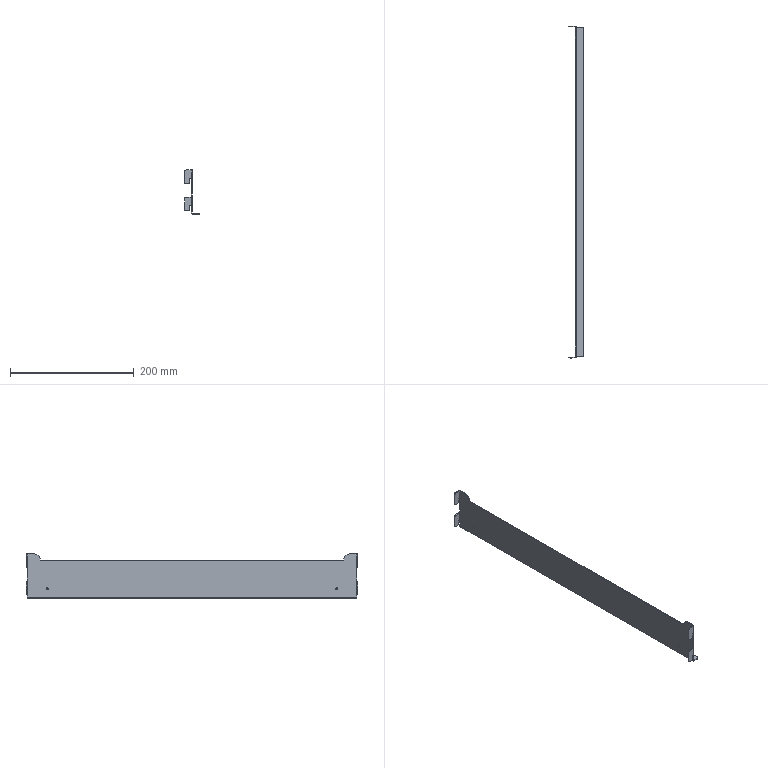Part | STEP file | RJWD-DY-0111_00 | 1 solid | 86 faces | box 24 x 537.5 x 71.5 mm | volume 60134 mm3 | plane 52 | cylinder 34 | commonest cylinder face diameters 6 x14 0.4 x5 3.4 x5 2 x4 3 x4 20 x2